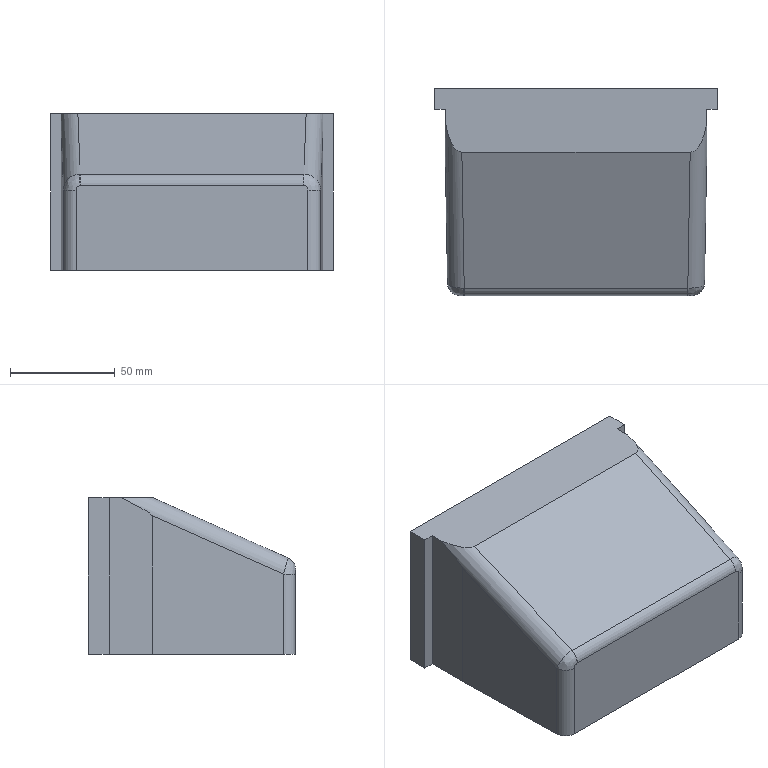Part | STEP file | 1 solid | 30 faces | box 135 x 99.045 x 75 mm | volume 726805 mm3 | plane 18 | cylinder 9 | spline 3 | commonest cylinder face diameters 16 x6 12 x3